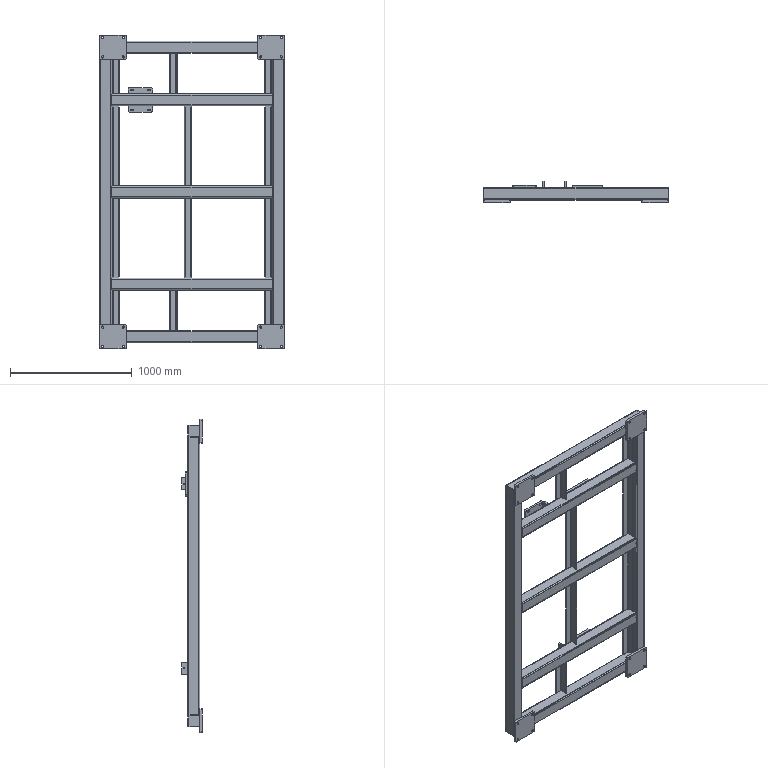Part | STEP file | 33 solids | 426 faces | box 1520 x 170 x 2580 mm | volume 30934372 mm3 | plane 234 | cylinder 192 | commonest cylinder face diameters 10 x50 20 x48 14 x32 18 x32 12 x24 8.5 x6